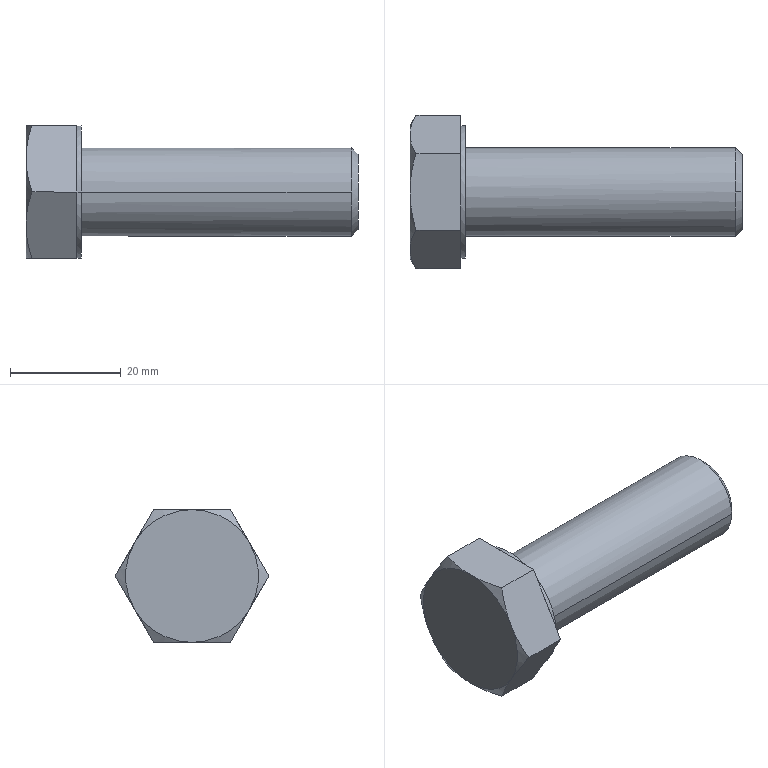Part | SolidWorks | features BaseBody 1 | 1 solid | 27 faces | box 60 x 27.713 x 24 mm | volume 14953 mm3 | plane 15 | cone 8 | cylinder 4 | commonest cylinder face diameters 16 x2 24 x2
STEP:
#1=CARTESIAN_POINT('',(0.,8.,0.));
#2=VERTEX_POINT('',#1);
#3=CARTESIAN_POINT('',(0.,-8.,0.));
#4=VERTEX_POINT('',#3);
#5=CARTESIAN_POINT('',(0.,0.,0.));
#6=DIRECTION('',(1.,0.,0.));
#7=DIRECTION('',(0.,1.,0.));
#8=AXIS2_PLACEMENT_3D('',#5,#6,#7);
#9=CIRCLE('',#8,8.);
#10=EDGE_CURVE('',#2,#4,#9,.T.);
#11=ORIENTED_EDGE('',*,*,#10,.T.);
#12=CARTESIAN_POINT('',(48.773,-8.,0.));
#13=VERTEX_POINT('',#12);
#14=CARTESIAN_POINT('',(28.,-8.,0.));
#15=DIRECTION('',(1.,0.,0.));
#16=VECTOR('',#15,1000.);
#17=LINE('',#14,#16);
#18=EDGE_CURVE('',#4,#13,#17,.T.);
#19=ORIENTED_EDGE('',*,*,#18,.T.);
#20=CARTESIAN_POINT('',(48.773,0.,8.));
#21=VERTEX_POINT('',#20);
#22=CARTESIAN_POINT('',(48.773,0.,0.));
#23=DIRECTION('',(-1.,0.,0.));
#24=DIRECTION('',(0.,1.,0.));
#25=AXIS2_PLACEMENT_3D('',#22,#23,#24);
#26=CIRCLE('',#25,8.);
#27=EDGE_CURVE('',#13,#21,#26,.T.);
#28=ORIENTED_EDGE('',*,*,#27,.T.);
#29=CARTESIAN_POINT('',(48.773,8.,0.));
#30=VERTEX_POINT('',#29);
#31=CARTESIAN_POINT('',(48.773,0.,0.));
#32=DIRECTION('',(-1.,0.,0.));
#33=DIRECTION('',(0.,1.,0.));
#34=AXIS2_PLACEMENT_3D('',#31,#32,#33);
#35=CIRCLE('',#34,8.);
#36=EDGE_CURVE('',#21,#30,#35,.T.);
#37=ORIENTED_EDGE('',*,*,#36,.T.);
#38=CARTESIAN_POINT('',(28.,8.,0.));
#39=DIRECTION('',(1.,0.,0.));
#40=VECTOR('',#39,1000.);
#41=LINE('',#38,#40);
#42=EDGE_CURVE('',#2,#30,#41,.T.);
#43=ORIENTED_EDGE('',*,*,#42,.F.);
#44=EDGE_LOOP('',(#11,#19,#28,#37,#43));
#45=FACE_OUTER_BOUND('',#44,.T.);
#46=CARTESIAN_POINT('',(28.,0.,0.));
#47=DIRECTION('',(1.,0.,0.));
#48=DIRECTION('',(0.,1.,0.));
#49=AXIS2_PLACEMENT_3D('',#46,#47,#48);
#50=CYLINDRICAL_SURFACE('',#49,8.);
#51=ADVANCED_FACE('',(#45),#50,.T.);
#52=CARTESIAN_POINT('',(50.,0.,6.773));
#53=VERTEX_POINT('',#52);
#54=CARTESIAN_POINT('',(50.,0.,-6.773));
#55=VERTEX_POINT('',#54);
#56=CARTESIAN_POINT('',(50.,0.,0.));
#57=DIRECTION('',(-1.,0.,0.));
#58=DIRECTION('',(0.,0.,1.));
#59=AXIS2_PLACEMENT_3D('',#56,#57,#58);
#60=CIRCLE('',#59,6.773);
#61=EDGE_CURVE('',#53,#55,#60,.T.);
#62=ORIENTED_EDGE('',*,*,#61,.T.);
#63=CARTESIAN_POINT('',(48.773,0.,-8.));
#64=VERTEX_POINT('',#63);
#65=CARTESIAN_POINT('',(48.773,0.,-8.));
#66=DIRECTION('',(-0.7071,0.,-0.7071));
#67=VECTOR('',#66,1000.);
#68=LINE('',#65,#67);
#69=EDGE_CURVE('',#55,#64,#68,.T.);
#70=ORIENTED_EDGE('',*,*,#69,.T.);
#71=CARTESIAN_POINT('',(48.773,0.,0.));
#72=DIRECTION('',(-1.,0.,0.));
#73=DIRECTION('',(0.,1.,0.));
#74=AXIS2_PLACEMENT_3D('',#71,#72,#73);
#75=CIRCLE('',#74,8.);
#76=EDGE_CURVE('',#30,#64,#75,.T.);
#77=ORIENTED_EDGE('',*,*,#76,.F.);
#78=ORIENTED_EDGE('',*,*,#36,.F.);
#79=CARTESIAN_POINT('',(48.773,0.,8.));
#80=DIRECTION('',(-0.7071,0.,0.7071));
#81=VECTOR('',#80,1000.);
#82=LINE('',#79,#81);
#83=EDGE_CURVE('',#53,#21,#82,.T.);
#84=ORIENTED_EDGE('',*,*,#83,.F.);
#85=EDGE_LOOP('',(#62,#70,#77,#78,#84));
#86=FACE_OUTER_BOUND('',#85,.T.);
#87=CARTESIAN_POINT('',(48.773,0.,0.));
#88=DIRECTION('',(-1.,0.,0.));
#89=DIRECTION('',(0.,0.,1.));
#90=AXIS2_PLACEMENT_3D('',#87,#88,#89);
#91=CONICAL_SURFACE('',#90,8.,0.7854);
#92=ADVANCED_FACE('',(#86),#91,.T.);
#93=CARTESIAN_POINT('',(-0.8001,-10.392,6.));
#94=VERTEX_POINT('',#93);
#95=CARTESIAN_POINT('',(-0.8001,-12.,0.));
#96=VERTEX_POINT('',#95);
#97=CARTESIAN_POINT('',(-0.8001,0.,0.));
#98=DIRECTION('',(1.,0.,0.));
#99=DIRECTION('',(0.,1.,0.));
#100=AXIS2_PLACEMENT_3D('',#97,#98,#99);
#101=CIRCLE('',#100,12.);
#102=EDGE_CURVE('',#94,#96,#101,.T.);
#103=ORIENTED_EDGE('',*,*,#102,.T.);
#104=CARTESIAN_POINT('',(0.,-12.,0.));
#105=VERTEX_POINT('',#104);
#106=CARTESIAN_POINT('',(-0.4,-12.,0.));
#107=DIRECTION('',(1.,0.,0.));
#108=VECTOR('',#107,1000.);
#109=LINE('',#106,#108);
#110=EDGE_CURVE('',#96,#105,#109,.T.);
#111=ORIENTED_EDGE('',*,*,#110,.T.);
#112=CARTESIAN_POINT('',(0.,12.,0.));
#113=VERTEX_POINT('',#112);
#114=CARTESIAN_POINT('',(0.,0.,0.));
#115=DIRECTION('',(1.,0.,0.));
#116=DIRECTION('',(0.,1.,0.));
#117=AXIS2_PLACEMENT_3D('',#114,#115,#116);
#118=CIRCLE('',#117,12.);
#119=EDGE_CURVE('',#113,#105,#118,.T.);
#120=ORIENTED_EDGE('',*,*,#119,.F.);
#121=CARTESIAN_POINT('',(-0.8001,12.,0.));
#122=VERTEX_POINT('',#121);
#123=CARTESIAN_POINT('',(-0.4,12.,0.));
#124=DIRECTION('',(1.,0.,0.));
#125=VECTOR('',#124,1000.);
#126=LINE('',#123,#125);
#127=EDGE_CURVE('',#122,#113,#126,.T.);
#128=ORIENTED_EDGE('',*,*,#127,.F.);
#129=CARTESIAN_POINT('',(-0.8001,10.392,6.));
#130=VERTEX_POINT('',#129);
#131=CARTESIAN_POINT('',(-0.8001,0.,0.));
#132=DIRECTION('',(1.,0.,0.));
#133=DIRECTION('',(0.,1.,0.));
#134=AXIS2_PLACEMENT_3D('',#131,#132,#133);
#135=CIRCLE('',#134,12.);
#136=EDGE_CURVE('',#122,#130,#135,.T.);
#137=ORIENTED_EDGE('',*,*,#136,.T.);
#138=CARTESIAN_POINT('',(-0.8001,0.,12.));
#139=VERTEX_POINT('',#138);
#140=CARTESIAN_POINT('',(-0.8001,0.,0.));
#141=DIRECTION('',(1.,0.,0.));
#142=DIRECTION('',(0.,1.,0.));
#143=AXIS2_PLACEMENT_3D('',#140,#141,#142);
#144=CIRCLE('',#143,12.);
#145=EDGE_CURVE('',#130,#139,#144,.T.);
#146=ORIENTED_EDGE('',*,*,#145,.T.);
#147=CARTESIAN_POINT('',(-0.8001,0.,0.));
#148=DIRECTION('',(1.,0.,0.));
#149=DIRECTION('',(0.,1.,0.));
#150=AXIS2_PLACEMENT_3D('',#147,#148,#149);
#151=CIRCLE('',#150,12.);
#152=EDGE_CURVE('',#139,#94,#151,.T.);
#153=ORIENTED_EDGE('',*,*,#152,.T.);
#154=EDGE_LOOP('',(#103,#111,#120,#128,#137,#146,#153));
#155=FACE_OUTER_BOUND('',#154,.T.);
#156=CARTESIAN_POINT('',(-0.4,0.,0.));
#157=DIRECTION('',(1.,0.,0.));
#158=DIRECTION('',(0.,1.,0.));
#159=AXIS2_PLACEMENT_3D('',#156,#157,#158);
#160=CYLINDRICAL_SURFACE('',#159,12.);
#161=ADVANCED_FACE('',(#155),#160,.T.);
#162=ORIENTED_EDGE('',*,*,#18,.F.);
#163=CARTESIAN_POINT('',(0.,0.,0.));
#164=DIRECTION('',(1.,0.,0.));
#165=DIRECTION('',(0.,1.,0.));
#166=AXIS2_PLACEMENT_3D('',#163,#164,#165);
#167=CIRCLE('',#166,8.);
#168=EDGE_CURVE('',#4,#2,#167,.T.);
#169=ORIENTED_EDGE('',*,*,#168,.T.);
#170=ORIENTED_EDGE('',*,*,#42,.T.);
#171=ORIENTED_EDGE('',*,*,#76,.T.);
#172=CARTESIAN_POINT('',(48.773,0.,0.));
#173=DIRECTION('',(-1.,0.,0.));
#174=DIRECTION('',(0.,1.,0.));
#175=AXIS2_PLACEMENT_3D('',#172,#173,#174);
#176=CIRCLE('',#175,8.);
#177=EDGE_CURVE('',#64,#13,#176,.T.);
#178=ORIENTED_EDGE('',*,*,#177,.T.);
#179=EDGE_LOOP('',(#162,#169,#170,#171,#178));
#180=FACE_OUTER_BOUND('',#179,.T.);
#181=CARTESIAN_POINT('',(28.,0.,0.));
#182=DIRECTION('',(1.,0.,0.));
#183=DIRECTION('',(0.,1.,0.));
#184=AXIS2_PLACEMENT_3D('',#181,#182,#183);
#185=CYLINDRICAL_SURFACE('',#184,8.);
#186=ADVANCED_FACE('',(#180),#185,.T.);
#187=ORIENTED_EDGE('',*,*,#69,.F.);
#188=CARTESIAN_POINT('',(50.,0.,0.));
#189=DIRECTION('',(-1.,0.,0.));
#190=DIRECTION('',(0.,0.,1.));
#191=AXIS2_PLACEMENT_3D('',#188,#189,#190);
#192=CIRCLE('',#191,6.773);
#193=EDGE_CURVE('',#55,#53,#192,.T.);
#194=ORIENTED_EDGE('',*,*,#193,.T.);
#195=ORIENTED_EDGE('',*,*,#83,.T.);
#196=ORIENTED_EDGE('',*,*,#27,.F.);
#197=ORIENTED_EDGE('',*,*,#177,.F.);
#198=EDGE_LOOP('',(#187,#194,#195,#196,#197));
#199=FACE_OUTER_BOUND('',#198,.T.);
#200=CARTESIAN_POINT('',(48.773,0.,0.));
#201=DIRECTION('',(-1.,0.,0.));
#202=DIRECTION('',(0.,0.,1.));
#203=AXIS2_PLACEMENT_3D('',#200,#201,#202);
#204=CONICAL_SURFACE('',#203,8.,0.7854);
#205=ADVANCED_FACE('',(#199),#204,.T.);
#206=ORIENTED_EDGE('',*,*,#10,.F.);
#207=ORIENTED_EDGE('',*,*,#168,.F.);
#208=EDGE_LOOP('',(#206,#207));
#209=FACE_BOUND('',#208,.T.);
#210=ORIENTED_EDGE('',*,*,#119,.T.);
#211=CARTESIAN_POINT('',(0.,0.,0.));
#212=DIRECTION('',(1.,0.,0.));
#213=DIRECTION('',(0.,1.,0.));
#214=AXIS2_PLACEMENT_3D('',#211,#212,#213);
#215=CIRCLE('',#214,12.);
#216=EDGE_CURVE('',#105,#113,#215,.T.);
#217=ORIENTED_EDGE('',*,*,#216,.T.);
#218=EDGE_LOOP('',(#210,#217));
#219=FACE_OUTER_BOUND('',#218,.T.);
#220=CARTESIAN_POINT('',(0.,10.,0.));
#221=DIRECTION('',(1.,0.,0.));
#222=DIRECTION('',(0.,1.,0.));
#223=AXIS2_PLACEMENT_3D('',#220,#221,#222);
#224=PLANE('',#223);
#225=ADVANCED_FACE('',(#209,#219),#224,.T.);
#226=ORIENTED_EDGE('',*,*,#61,.F.);
#227=ORIENTED_EDGE('',*,*,#193,.F.);
#228=EDGE_LOOP('',(#226,#227));
#229=FACE_OUTER_BOUND('',#228,.T.);
#230=CARTESIAN_POINT('',(50.,4.,0.));
#231=DIRECTION('',(1.,0.,0.));
#232=DIRECTION('',(0.,1.,0.));
#233=AXIS2_PLACEMENT_3D('',#230,#231,#232);
#234=PLANE('',#233);
#235=ADVANCED_FACE('',(#229),#234,.T.);
#236=ORIENTED_EDGE('',*,*,#110,.F.);
#237=CARTESIAN_POINT('',(-0.8001,-10.392,-6.));
#238=VERTEX_POINT('',#237);
#239=CARTESIAN_POINT('',(-0.8001,0.,0.));
#240=DIRECTION('',(1.,0.,0.));
#241=DIRECTION('',(0.,1.,0.));
#242=AXIS2_PLACEMENT_3D('',#239,#240,#241);
#243=CIRCLE('',#242,12.);
#244=EDGE_CURVE('',#96,#238,#243,.T.);
#245=ORIENTED_EDGE('',*,*,#244,.T.);
#246=CARTESIAN_POINT('',(-0.8001,0.,-12.));
#247=VERTEX_POINT('',#246);
#248=CARTESIAN_POINT('',(-0.8001,0.,0.));
#249=DIRECTION('',(1.,0.,0.));
#250=DIRECTION('',(0.,1.,0.));
#251=AXIS2_PLACEMENT_3D('',#248,#249,#250);
#252=CIRCLE('',#251,12.);
#253=EDGE_CURVE('',#238,#247,#252,.T.);
#254=ORIENTED_EDGE('',*,*,#253,.T.);
#255=CARTESIAN_POINT('',(-0.8001,10.392,-6.));
#256=VERTEX_POINT('',#255);
#257=CARTESIAN_POINT('',(-0.8001,0.,0.));
#258=DIRECTION('',(1.,0.,0.));
#259=DIRECTION('',(0.,1.,0.));
#260=AXIS2_PLACEMENT_3D('',#257,#258,#259);
#261=CIRCLE('',#260,12.);
#262=EDGE_CURVE('',#247,#256,#261,.T.);
#263=ORIENTED_EDGE('',*,*,#262,.T.);
#264=CARTESIAN_POINT('',(-0.8001,0.,0.));
#265=DIRECTION('',(1.,0.,0.));
#266=DIRECTION('',(0.,1.,0.));
#267=AXIS2_PLACEMENT_3D('',#264,#265,#266);
#268=CIRCLE('',#267,12.);
#269=EDGE_CURVE('',#256,#122,#268,.T.);
#270=ORIENTED_EDGE('',*,*,#269,.T.);
#271=ORIENTED_EDGE('',*,*,#127,.T.);
#272=ORIENTED_EDGE('',*,*,#216,.F.);
#273=EDGE_LOOP('',(#236,#245,#254,#263,#270,#271,#272));
#274=FACE_OUTER_BOUND('',#273,.T.);
#275=CARTESIAN_POINT('',(-0.4,0.,0.));
#276=DIRECTION('',(1.,0.,0.));
#277=DIRECTION('',(0.,1.,0.));
#278=AXIS2_PLACEMENT_3D('',#275,#276,#277);
#279=CYLINDRICAL_SURFACE('',#278,12.);
#280=ADVANCED_FACE('',(#274),#279,.T.);
#281=CARTESIAN_POINT('',(-0.8001,6.928,-12.));
#282=VERTEX_POINT('',#281);
#283=CARTESIAN_POINT('',(-0.8001,0.,-12.));
#284=DIRECTION('',(0.,1.,0.));
#285=VECTOR('',#284,1000.);
#286=LINE('',#283,#285);
#287=EDGE_CURVE('',#247,#282,#286,.T.);
#288=ORIENTED_EDGE('',*,*,#287,.T.);
#289=CARTESIAN_POINT('',(-0.8001,6.928,-12.));
#290=DIRECTION('',(0.,0.5,0.866));
#291=VECTOR('',#290,1000.);
#292=LINE('',#289,#291);
#293=EDGE_CURVE('',#282,#256,#292,.T.);
#294=ORIENTED_EDGE('',*,*,#293,.T.);
#295=ORIENTED_EDGE('',*,*,#262,.F.);
#296=EDGE_LOOP('',(#288,#294,#295));
#297=FACE_OUTER_BOUND('',#296,.T.);
#298=CARTESIAN_POINT('',(-0.8001,0.,0.));
#299=DIRECTION('',(1.,0.,0.));
#300=DIRECTION('',(0.,1.,0.));
#301=AXIS2_PLACEMENT_3D('',#298,#299,#300);
#302=PLANE('',#301);
#303=ADVANCED_FACE('',(#297),#302,.T.);
#304=CARTESIAN_POINT('',(-0.8001,-6.928,-12.));
#305=VERTEX_POINT('',#304);
#306=CARTESIAN_POINT('',(-0.8001,-10.392,-6.));
#307=DIRECTION('',(0.,0.5,-0.866));
#308=VECTOR('',#307,1000.);
#309=LINE('',#306,#308);
#310=EDGE_CURVE('',#238,#305,#309,.T.);
#311=ORIENTED_EDGE('',*,*,#310,.T.);
#312=CARTESIAN_POINT('',(-0.8001,0.,-12.));
#313=DIRECTION('',(0.,1.,0.));
#314=VECTOR('',#313,1000.);
#315=LINE('',#312,#314);
#316=EDGE_CURVE('',#305,#247,#315,.T.);
#317=ORIENTED_EDGE('',*,*,#316,.T.);
#318=ORIENTED_EDGE('',*,*,#253,.F.);
#319=EDGE_LOOP('',(#311,#317,#318));
#320=FACE_OUTER_BOUND('',#319,.T.);
#321=CARTESIAN_POINT('',(-0.8001,0.,0.));
#322=DIRECTION('',(1.,0.,0.));
#323=DIRECTION('',(0.,1.,0.));
#324=AXIS2_PLACEMENT_3D('',#321,#322,#323);
#325=PLANE('',#324);
#326=ADVANCED_FACE('',(#320),#325,.T.);
#327=CARTESIAN_POINT('',(-0.8001,-13.856,0.));
#328=VERTEX_POINT('',#327);
#329=CARTESIAN_POINT('',(-0.8001,-10.392,6.));
#330=DIRECTION('',(0.,-0.5,-0.866));
#331=VECTOR('',#330,1000.);
#332=LINE('',#329,#331);
#333=EDGE_CURVE('',#94,#328,#332,.T.);
#334=ORIENTED_EDGE('',*,*,#333,.T.);
#335=CARTESIAN_POINT('',(-0.8001,-13.856,0.));
#336=DIRECTION('',(0.,0.5,-0.866));
#337=VECTOR('',#336,1000.);
#338=LINE('',#335,#337);
#339=EDGE_CURVE('',#328,#238,#338,.T.);
#340=ORIENTED_EDGE('',*,*,#339,.T.);
#341=ORIENTED_EDGE('',*,*,#244,.F.);
#342=ORIENTED_EDGE('',*,*,#102,.F.);
#343=EDGE_LOOP('',(#334,#340,#341,#342));
#344=FACE_OUTER_BOUND('',#343,.T.);
#345=CARTESIAN_POINT('',(-0.8001,0.,0.));
#346=DIRECTION('',(1.,0.,0.));
#347=DIRECTION('',(0.,1.,0.));
#348=AXIS2_PLACEMENT_3D('',#345,#346,#347);
#349=PLANE('',#348);
#350=ADVANCED_FACE('',(#344),#349,.T.);
#351=CARTESIAN_POINT('',(-0.8001,-6.928,12.));
#352=VERTEX_POINT('',#351);
#353=CARTESIAN_POINT('',(-0.8001,0.,12.));
#354=DIRECTION('',(0.,-1.,0.));
#355=VECTOR('',#354,1000.);
#356=LINE('',#353,#355);
#357=EDGE_CURVE('',#139,#352,#356,.T.);
#358=ORIENTED_EDGE('',*,*,#357,.T.);
#359=CARTESIAN_POINT('',(-0.8001,-6.928,12.));
#360=DIRECTION('',(0.,-0.5,-0.866));
#361=VECTOR('',#360,1000.);
#362=LINE('',#359,#361);
#363=EDGE_CURVE('',#352,#94,#362,.T.);
#364=ORIENTED_EDGE('',*,*,#363,.T.);
#365=ORIENTED_EDGE('',*,*,#152,.F.);
#366=EDGE_LOOP('',(#358,#364,#365));
#367=FACE_OUTER_BOUND('',#366,.T.);
#368=CARTESIAN_POINT('',(-0.8001,0.,0.));
#369=DIRECTION('',(1.,0.,0.));
#370=DIRECTION('',(0.,1.,0.));
#371=AXIS2_PLACEMENT_3D('',#368,#369,#370);
#372=PLANE('',#371);
#373=ADVANCED_FACE('',(#367),#372,.T.);
#374=CARTESIAN_POINT('',(-0.8001,6.928,12.));
#375=VERTEX_POINT('',#374);
#376=CARTESIAN_POINT('',(-0.8001,10.392,6.));
#377=DIRECTION('',(0.,-0.5,0.866));
#378=VECTOR('',#377,1000.);
#379=LINE('',#376,#378);
#380=EDGE_CURVE('',#130,#375,#379,.T.);
#381=ORIENTED_EDGE('',*,*,#380,.T.);
#382=CARTESIAN_POINT('',(-0.8001,0.,12.));
#383=DIRECTION('',(0.,-1.,0.));
#384=VECTOR('',#383,1000.);
#385=LINE('',#382,#384);
#386=EDGE_CURVE('',#375,#139,#385,.T.);
#387=ORIENTED_EDGE('',*,*,#386,.T.);
#388=ORIENTED_EDGE('',*,*,#145,.F.);
#389=EDGE_LOOP('',(#381,#387,#388));
#390=FACE_OUTER_BOUND('',#389,.T.);
#391=CARTESIAN_POINT('',(-0.8001,0.,0.));
#392=DIRECTION('',(1.,0.,0.));
#393=DIRECTION('',(0.,1.,0.));
#394=AXIS2_PLACEMENT_3D('',#391,#392,#393);
#395=PLANE('',#394);
#396=ADVANCED_FACE('',(#390),#395,.T.);
#397=CARTESIAN_POINT('',(-0.8001,13.856,0.));
#398=VERTEX_POINT('',#397);
#399=CARTESIAN_POINT('',(-0.8001,10.392,-6.));
#400=DIRECTION('',(0.,0.5,0.866));
#401=VECTOR('',#400,1000.);
#402=LINE('',#399,#401);
#403=EDGE_CURVE('',#256,#398,#402,.T.);
#404=ORIENTED_EDGE('',*,*,#403,.T.);
#405=CARTESIAN_POINT('',(-0.8001,13.856,0.));
#406=DIRECTION('',(0.,-0.5,0.866));
#407=VECTOR('',#406,1000.);
#408=LINE('',#405,#407);
#409=EDGE_CURVE('',#398,#130,#408,.T.);
#410=ORIENTED_EDGE('',*,*,#409,.T.);
#411=ORIENTED_EDGE('',*,*,#136,.F.);
#412=ORIENTED_EDGE('',*,*,#269,.F.);
#413=EDGE_LOOP('',(#404,#410,#411,#412));
#414=FACE_OUTER_BOUND('',#413,.T.);
#415=CARTESIAN_POINT('',(-0.8001,0.,0.));
#416=DIRECTION('',(1.,0.,0.));
#417=DIRECTION('',(0.,1.,0.));
#418=AXIS2_PLACEMENT_3D('',#415,#416,#417);
#419=PLANE('',#418);
#420=ADVANCED_FACE('',(#414),#419,.T.);
#421=ORIENTED_EDGE('',*,*,#293,.F.);
#422=CARTESIAN_POINT('',(-8.928,6.928,-12.));
#423=VERTEX_POINT('',#422);
#424=CARTESIAN_POINT('',(-0.8001,6.928,-12.));
#425=DIRECTION('',(-1.,0.,0.));
#426=VECTOR('',#425,1000.);
#427=LINE('',#424,#426);
#428=EDGE_CURVE('',#282,#423,#427,.T.);
#429=ORIENTED_EDGE('',*,*,#428,.T.);
#430=CARTESIAN_POINT('',(-10.,10.392,-6.));
#431=VERTEX_POINT('',#430);
#432=CARTESIAN_POINT('',(-8.928,6.928,-12.));
#433=CARTESIAN_POINT('',(-9.255,7.494,-11.02));
#434=CARTESIAN_POINT('',(-9.524,8.064,-10.032));
#435=CARTESIAN_POINT('',(-9.898,9.218,-8.034));
#436=CARTESIAN_POINT('',(-10.,9.801,-7.024));
#437=CARTESIAN_POINT('',(-10.,10.392,-6.));
#438=B_SPLINE_CURVE_WITH_KNOTS('',3,(#432,#433,#434,#435,#436,#437),.UNSPECIFIED.,.F.,.F.,(4,2,4),(0.,0.003505,0.007011),.UNSPECIFIED.);
#439=EDGE_CURVE('',#423,#431,#438,.T.);
#440=ORIENTED_EDGE('',*,*,#439,.T.);
#441=CARTESIAN_POINT('',(-8.928,13.856,0.));
#442=VERTEX_POINT('',#441);
#443=CARTESIAN_POINT('',(-10.,10.392,-6.));
#444=CARTESIAN_POINT('',(-10.,10.983,-4.976));
#445=CARTESIAN_POINT('',(-9.898,11.567,-3.966));
#446=CARTESIAN_POINT('',(-9.524,12.72,-1.968));
#447=CARTESIAN_POINT('',(-9.255,13.291,-0.9802));
#448=CARTESIAN_POINT('',(-8.928,13.856,0.));
#449=B_SPLINE_CURVE_WITH_KNOTS('',3,(#443,#444,#445,#446,#447,#448),.UNSPECIFIED.,.F.,.F.,(4,2,4),(0.,0.003505,0.007011),.UNSPECIFIED.);
#450=EDGE_CURVE('',#431,#442,#449,.T.);
#451=ORIENTED_EDGE('',*,*,#450,.T.);
#452=CARTESIAN_POINT('',(-0.8001,13.856,0.));
#453=DIRECTION('',(1.,0.,0.));
#454=VECTOR('',#453,1000.);
#455=LINE('',#452,#454);
#456=EDGE_CURVE('',#442,#398,#455,.T.);
#457=ORIENTED_EDGE('',*,*,#456,.T.);
#458=ORIENTED_EDGE('',*,*,#403,.F.);
#459=EDGE_LOOP('',(#421,#429,#440,#451,#457,#458));
#460=FACE_OUTER_BOUND('',#459,.T.);
#461=CARTESIAN_POINT('',(-0.8001,6.928,-12.));
#462=DIRECTION('',(0.,0.866,-0.5));
#463=DIRECTION('',(0.,0.5,0.866));
#464=AXIS2_PLACEMENT_3D('',#461,#462,#463);
#465=PLANE('',#464);
#466=ADVANCED_FACE('',(#460),#465,.T.);
#467=ORIENTED_EDGE('',*,*,#316,.F.);
#468=CARTESIAN_POINT('',(-8.928,-6.928,-12.));
#469=VERTEX_POINT('',#468);
#470=CARTESIAN_POINT('',(-0.8001,-6.928,-12.));
#471=DIRECTION('',(-1.,0.,0.));
#472=VECTOR('',#471,1000.);
#473=LINE('',#470,#472);
#474=EDGE_CURVE('',#305,#469,#473,.T.);
#475=ORIENTED_EDGE('',*,*,#474,.T.);
#476=CARTESIAN_POINT('',(-10.,0.,-12.));
#477=VERTEX_POINT('',#476);
#478=CARTESIAN_POINT('',(-8.928,-6.928,-12.));
#479=CARTESIAN_POINT('',(-9.255,-5.796,-12.));
#480=CARTESIAN_POINT('',(-9.524,-4.656,-12.));
#481=CARTESIAN_POINT('',(-9.898,-2.349,-12.));
#482=CARTESIAN_POINT('',(-10.,-1.182,-12.));
#483=CARTESIAN_POINT('',(-10.,0.,-12.));
#484=B_SPLINE_CURVE_WITH_KNOTS('',3,(#478,#479,#480,#481,#482,#483),.UNSPECIFIED.,.F.,.F.,(4,2,4),(0.,0.003505,0.007011),.UNSPECIFIED.);
#485=EDGE_CURVE('',#469,#477,#484,.T.);
#486=ORIENTED_EDGE('',*,*,#485,.T.);
#487=CARTESIAN_POINT('',(-10.,0.,-12.));
#488=CARTESIAN_POINT('',(-10.,1.182,-12.));
#489=CARTESIAN_POINT('',(-9.898,2.349,-12.));
#490=CARTESIAN_POINT('',(-9.524,4.656,-12.));
#491=CARTESIAN_POINT('',(-9.255,5.796,-12.));
#492=CARTESIAN_POINT('',(-8.928,6.928,-12.));
#493=B_SPLINE_CURVE_WITH_KNOTS('',3,(#487,#488,#489,#490,#491,#492),.UNSPECIFIED.,.F.,.F.,(4,2,4),(0.,0.003505,0.007011),.UNSPECIFIED.);
#494=EDGE_CURVE('',#477,#423,#493,.T.);
#495=ORIENTED_EDGE('',*,*,#494,.T.);
#496=ORIENTED_EDGE('',*,*,#428,.F.);
#497=ORIENTED_EDGE('',*,*,#287,.F.);
#498=EDGE_LOOP('',(#467,#475,#486,#495,#496,#497));
#499=FACE_OUTER_BOUND('',#498,.T.);
#500=CARTESIAN_POINT('',(-0.8001,-6.928,-12.));
#501=DIRECTION('',(0.,0.,-1.));
#502=DIRECTION('',(0.,1.,0.));
#503=AXIS2_PLACEMENT_3D('',#500,#501,#502);
#504=PLANE('',#503);
#505=ADVANCED_FACE('',(#499),#504,.T.);
#506=CARTESIAN_POINT('',(-8.928,-13.856,0.));
#507=VERTEX_POINT('',#506);
#508=CARTESIAN_POINT('',(-0.8001,-13.856,0.));
#509=DIRECTION('',(-1.,0.,0.));
#510=VECTOR('',#509,1000.);
#511=LINE('',#508,#510);
#512=EDGE_CURVE('',#328,#507,#511,.T.);
#513=ORIENTED_EDGE('',*,*,#512,.T.);
#514=CARTESIAN_POINT('',(-10.,-10.392,-6.));
#515=VERTEX_POINT('',#514);
#516=CARTESIAN_POINT('',(-8.928,-13.856,0.));
#517=CARTESIAN_POINT('',(-9.255,-13.291,-0.9802));
#518=CARTESIAN_POINT('',(-9.524,-12.72,-1.968));
#519=CARTESIAN_POINT('',(-9.898,-11.567,-3.966));
#520=CARTESIAN_POINT('',(-10.,-10.983,-4.976));
#521=CARTESIAN_POINT('',(-10.,-10.392,-6.));
#522=B_SPLINE_CURVE_WITH_KNOTS('',3,(#516,#517,#518,#519,#520,#521),.UNSPECIFIED.,.F.,.F.,(4,2,4),(0.,0.003505,0.007011),.UNSPECIFIED.);
#523=EDGE_CURVE('',#507,#515,#522,.T.);
#524=ORIENTED_EDGE('',*,*,#523,.T.);
#525=CARTESIAN_POINT('',(-10.,-10.392,-6.));
#526=CARTESIAN_POINT('',(-10.,-9.801,-7.024));
#527=CARTESIAN_POINT('',(-9.898,-9.218,-8.034));
#528=CARTESIAN_POINT('',(-9.524,-8.064,-10.032));
#529=CARTESIAN_POINT('',(-9.255,-7.494,-11.02));
#530=CARTESIAN_POINT('',(-8.928,-6.928,-12.));
#531=B_SPLINE_CURVE_WITH_KNOTS('',3,(#525,#526,#527,#528,#529,#530),.UNSPECIFIED.,.F.,.F.,(4,2,4),(0.,0.003505,0.007011),.UNSPECIFIED.);
#532=EDGE_CURVE('',#515,#469,#531,.T.);
#533=ORIENTED_EDGE('',*,*,#532,.T.);
#534=ORIENTED_EDGE('',*,*,#474,.F.);
#535=ORIENTED_EDGE('',*,*,#310,.F.);
#536=ORIENTED_EDGE('',*,*,#339,.F.);
#537=EDGE_LOOP('',(#513,#524,#533,#534,#535,#536));
#538=FACE_OUTER_BOUND('',#537,.T.);
#539=CARTESIAN_POINT('',(-0.8001,-13.856,0.));
#540=DIRECTION('',(0.,-0.866,-0.5));
#541=DIRECTION('',(0.,0.5,-0.866));
#542=AXIS2_PLACEMENT_3D('',#539,#540,#541);
#543=PLANE('',#542);
#544=ADVANCED_FACE('',(#538),#543,.T.);
#545=CARTESIAN_POINT('',(-8.928,-6.928,12.));
#546=VERTEX_POINT('',#545);
#547=CARTESIAN_POINT('',(-0.8001,-6.928,12.));
#548=DIRECTION('',(-1.,0.,0.));
#549=VECTOR('',#548,1000.);
#550=LINE('',#547,#549);
#551=EDGE_CURVE('',#352,#546,#550,.T.);
#552=ORIENTED_EDGE('',*,*,#551,.T.);
#553=CARTESIAN_POINT('',(-10.,-10.392,6.));
#554=VERTEX_POINT('',#553);
#555=CARTESIAN_POINT('',(-8.928,-6.928,12.));
#556=CARTESIAN_POINT('',(-9.255,-7.494,11.02));
#557=CARTESIAN_POINT('',(-9.524,-8.064,10.032));
#558=CARTESIAN_POINT('',(-9.898,-9.218,8.034));
#559=CARTESIAN_POINT('',(-10.,-9.801,7.024));
#560=CARTESIAN_POINT('',(-10.,-10.392,6.));
#561=B_SPLINE_CURVE_WITH_KNOTS('',3,(#555,#556,#557,#558,#559,#560),.UNSPECIFIED.,.F.,.F.,(4,2,4),(0.,0.003505,0.007011),.UNSPECIFIED.);
#562=EDGE_CURVE('',#546,#554,#561,.T.);
#563=ORIENTED_EDGE('',*,*,#562,.T.);
#564=CARTESIAN_POINT('',(-10.,-10.392,6.));
#565=CARTESIAN_POINT('',(-10.,-10.983,4.976));
#566=CARTESIAN_POINT('',(-9.898,-11.567,3.966));
#567=CARTESIAN_POINT('',(-9.524,-12.72,1.968));
#568=CARTESIAN_POINT('',(-9.255,-13.291,0.9802));
#569=CARTESIAN_POINT('',(-8.928,-13.856,0.));
#570=B_SPLINE_CURVE_WITH_KNOTS('',3,(#564,#565,#566,#567,#568,#569),.UNSPECIFIED.,.F.,.F.,(4,2,4),(0.,0.003505,0.007011),.UNSPECIFIED.);
#571=EDGE_CURVE('',#554,#507,#570,.T.);
#572=ORIENTED_EDGE('',*,*,#571,.T.);
#573=ORIENTED_EDGE('',*,*,#512,.F.);
#574=ORIENTED_EDGE('',*,*,#333,.F.);
#575=ORIENTED_EDGE('',*,*,#363,.F.);
#576=EDGE_LOOP('',(#552,#563,#572,#573,#574,#575));
#577=FACE_OUTER_BOUND('',#576,.T.);
#578=CARTESIAN_POINT('',(-0.8001,-6.928,12.));
#579=DIRECTION('',(0.,-0.866,0.5));
#580=DIRECTION('',(0.,-0.5,-0.866));
#581=AXIS2_PLACEMENT_3D('',#578,#579,#580);
#582=PLANE('',#581);
#583=ADVANCED_FACE('',(#577),#582,.T.);
#584=CARTESIAN_POINT('',(-8.928,6.928,12.));
#585=VERTEX_POINT('',#584);
#586=CARTESIAN_POINT('',(-0.8001,6.928,12.));
#587=DIRECTION('',(-1.,0.,0.));
#588=VECTOR('',#587,1000.);
#589=LINE('',#586,#588);
#590=EDGE_CURVE('',#375,#585,#589,.T.);
#591=ORIENTED_EDGE('',*,*,#590,.T.);
#592=CARTESIAN_POINT('',(-10.,0.,12.));
#593=VERTEX_POINT('',#592);
#594=CARTESIAN_POINT('',(-8.928,6.928,12.));
#595=CARTESIAN_POINT('',(-9.255,5.796,12.));
#596=CARTESIAN_POINT('',(-9.524,4.656,12.));
#597=CARTESIAN_POINT('',(-9.898,2.349,12.));
#598=CARTESIAN_POINT('',(-10.,1.182,12.));
#599=CARTESIAN_POINT('',(-10.,0.,12.));
#600=B_SPLINE_CURVE_WITH_KNOTS('',3,(#594,#595,#596,#597,#598,#599),.UNSPECIFIED.,.F.,.F.,(4,2,4),(0.,0.003505,0.007011),.UNSPECIFIED.);
#601=EDGE_CURVE('',#585,#593,#600,.T.);
#602=ORIENTED_EDGE('',*,*,#601,.T.);
#603=CARTESIAN_POINT('',(-10.,0.,12.));
#604=CARTESIAN_POINT('',(-10.,-1.182,12.));
#605=CARTESIAN_POINT('',(-9.898,-2.349,12.));
#606=CARTESIAN_POINT('',(-9.524,-4.656,12.));
#607=CARTESIAN_POINT('',(-9.255,-5.796,12.));
#608=CARTESIAN_POINT('',(-8.928,-6.928,12.));
#609=B_SPLINE_CURVE_WITH_KNOTS('',3,(#603,#604,#605,#606,#607,#608),.UNSPECIFIED.,.F.,.F.,(4,2,4),(0.,0.003505,0.007011),.UNSPECIFIED.);
#610=EDGE_CURVE('',#593,#546,#609,.T.);
#611=ORIENTED_EDGE('',*,*,#610,.T.);
#612=ORIENTED_EDGE('',*,*,#551,.F.);
#613=ORIENTED_EDGE('',*,*,#357,.F.);
#614=ORIENTED_EDGE('',*,*,#386,.F.);
#615=EDGE_LOOP('',(#591,#602,#611,#612,#613,#614));
#616=FACE_OUTER_BOUND('',#615,.T.);
#617=CARTESIAN_POINT('',(-0.8001,6.928,12.));
#618=DIRECTION('',(0.,0.,1.));
#619=DIRECTION('',(0.,-1.,0.));
#620=AXIS2_PLACEMENT_3D('',#617,#618,#619);
#621=PLANE('',#620);
#622=ADVANCED_FACE('',(#616),#621,.T.);
#623=ORIENTED_EDGE('',*,*,#409,.F.);
#624=ORIENTED_EDGE('',*,*,#456,.F.);
#625=CARTESIAN_POINT('',(-10.,10.392,6.));
#626=VERTEX_POINT('',#625);
#627=CARTESIAN_POINT('',(-8.928,13.856,0.));
#628=CARTESIAN_POINT('',(-9.255,13.291,0.9802));
#629=CARTESIAN_POINT('',(-9.524,12.72,1.968));
#630=CARTESIAN_POINT('',(-9.898,11.567,3.966));
#631=CARTESIAN_POINT('',(-10.,10.983,4.976));
#632=CARTESIAN_POINT('',(-10.,10.392,6.));
#633=B_SPLINE_CURVE_WITH_KNOTS('',3,(#627,#628,#629,#630,#631,#632),.UNSPECIFIED.,.F.,.F.,(4,2,4),(0.,0.003505,0.007011),.UNSPECIFIED.);
#634=EDGE_CURVE('',#442,#626,#633,.T.);
#635=ORIENTED_EDGE('',*,*,#634,.T.);
#636=CARTESIAN_POINT('',(-10.,10.392,6.));
#637=CARTESIAN_POINT('',(-10.,9.801,7.024));
#638=CARTESIAN_POINT('',(-9.898,9.218,8.034));
#639=CARTESIAN_POINT('',(-9.524,8.064,10.032));
#640=CARTESIAN_POINT('',(-9.255,7.494,11.02));
#641=CARTESIAN_POINT('',(-8.928,6.928,12.));
#642=B_SPLINE_CURVE_WITH_KNOTS('',3,(#636,#637,#638,#639,#640,#641),.UNSPECIFIED.,.F.,.F.,(4,2,4),(0.,0.003505,0.007011),.UNSPECIFIED.);
#643=EDGE_CURVE('',#626,#585,#642,.T.);
#644=ORIENTED_EDGE('',*,*,#643,.T.);
#645=ORIENTED_EDGE('',*,*,#590,.F.);
#646=ORIENTED_EDGE('',*,*,#380,.F.);
#647=EDGE_LOOP('',(#623,#624,#635,#644,#645,#646));
#648=FACE_OUTER_BOUND('',#647,.T.);
#649=CARTESIAN_POINT('',(-0.8001,13.856,0.));
#650=DIRECTION('',(0.,0.866,0.5));
#651=DIRECTION('',(0.,-0.5,0.866));
#652=AXIS2_PLACEMENT_3D('',#649,#650,#651);
#653=PLANE('',#652);
#654=ADVANCED_FACE('',(#648),#653,.T.);
#655=CARTESIAN_POINT('',(-10.,0.,0.));
#656=DIRECTION('',(1.,0.,0.));
#657=DIRECTION('',(0.,0.,-1.));
#658=AXIS2_PLACEMENT_3D('',#655,#656,#657);
#659=CIRCLE('',#658,12.);
#660=EDGE_CURVE('',#431,#626,#659,.T.);
#661=ORIENTED_EDGE('',*,*,#660,.T.);
#662=ORIENTED_EDGE('',*,*,#634,.F.);
#663=ORIENTED_EDGE('',*,*,#450,.F.);
#664=EDGE_LOOP('',(#661,#662,#663));
#665=FACE_OUTER_BOUND('',#664,.T.);
#666=CARTESIAN_POINT('',(-8.922,0.,0.));
#667=DIRECTION('',(1.,0.,0.));
#668=DIRECTION('',(0.,0.,-1.));
#669=AXIS2_PLACEMENT_3D('',#666,#667,#668);
#670=CONICAL_SURFACE('',#669,13.868,1.047);
#671=ADVANCED_FACE('',(#665),#670,.T.);
#672=CARTESIAN_POINT('',(-10.,0.,0.));
#673=DIRECTION('',(1.,0.,0.));
#674=DIRECTION('',(0.,0.,-1.));
#675=AXIS2_PLACEMENT_3D('',#672,#673,#674);
#676=CIRCLE('',#675,12.);
#677=EDGE_CURVE('',#477,#431,#676,.T.);
#678=ORIENTED_EDGE('',*,*,#677,.T.);
#679=ORIENTED_EDGE('',*,*,#439,.F.);
#680=ORIENTED_EDGE('',*,*,#494,.F.);
#681=EDGE_LOOP('',(#678,#679,#680));
#682=FACE_OUTER_BOUND('',#681,.T.);
#683=CARTESIAN_POINT('',(-8.922,0.,0.));
#684=DIRECTION('',(1.,0.,0.));
#685=DIRECTION('',(0.,0.,-1.));
#686=AXIS2_PLACEMENT_3D('',#683,#684,#685);
#687=CONICAL_SURFACE('',#686,13.868,1.047);
#688=ADVANCED_FACE('',(#682),#687,.T.);
#689=ORIENTED_EDGE('',*,*,#532,.F.);
#690=CARTESIAN_POINT('',(-10.,0.,0.));
#691=DIRECTION('',(1.,0.,0.));
#692=DIRECTION('',(0.,0.,-1.));
#693=AXIS2_PLACEMENT_3D('',#690,#691,#692);
#694=CIRCLE('',#693,12.);
#695=EDGE_CURVE('',#515,#477,#694,.T.);
#696=ORIENTED_EDGE('',*,*,#695,.T.);
#697=ORIENTED_EDGE('',*,*,#485,.F.);
#698=EDGE_LOOP('',(#689,#696,#697));
#699=FACE_OUTER_BOUND('',#698,.T.);
#700=CARTESIAN_POINT('',(-8.922,0.,0.));
#701=DIRECTION('',(1.,0.,0.));
#702=DIRECTION('',(0.,0.,-1.));
#703=AXIS2_PLACEMENT_3D('',#700,#701,#702);
#704=CONICAL_SURFACE('',#703,13.868,1.047);
#705=ADVANCED_FACE('',(#699),#704,.T.);
#706=ORIENTED_EDGE('',*,*,#571,.F.);
#707=CARTESIAN_POINT('',(-10.,0.,0.));
#708=DIRECTION('',(1.,0.,0.));
#709=DIRECTION('',(0.,0.,-1.));
#710=AXIS2_PLACEMENT_3D('',#707,#708,#709);
#711=CIRCLE('',#710,12.);
#712=EDGE_CURVE('',#554,#515,#711,.T.);
#713=ORIENTED_EDGE('',*,*,#712,.T.);
#714=ORIENTED_EDGE('',*,*,#523,.F.);
#715=EDGE_LOOP('',(#706,#713,#714));
#716=FACE_OUTER_BOUND('',#715,.T.);
#717=CARTESIAN_POINT('',(-8.922,0.,0.));
#718=DIRECTION('',(1.,0.,0.));
#719=DIRECTION('',(0.,0.,-1.));
#720=AXIS2_PLACEMENT_3D('',#717,#718,#719);
#721=CONICAL_SURFACE('',#720,13.868,1.047);
#722=ADVANCED_FACE('',(#716),#721,.T.);
#723=ORIENTED_EDGE('',*,*,#610,.F.);
#724=CARTESIAN_POINT('',(-10.,0.,0.));
#725=DIRECTION('',(1.,0.,0.));
#726=DIRECTION('',(0.,0.,-1.));
#727=AXIS2_PLACEMENT_3D('',#724,#725,#726);
#728=CIRCLE('',#727,12.);
#729=EDGE_CURVE('',#593,#554,#728,.T.);
#730=ORIENTED_EDGE('',*,*,#729,.T.);
#731=ORIENTED_EDGE('',*,*,#562,.F.);
#732=EDGE_LOOP('',(#723,#730,#731));
#733=FACE_OUTER_BOUND('',#732,.T.);
#734=CARTESIAN_POINT('',(-8.922,0.,0.));
#735=DIRECTION('',(1.,0.,0.));
#736=DIRECTION('',(0.,0.,-1.));
#737=AXIS2_PLACEMENT_3D('',#734,#735,#736);
#738=CONICAL_SURFACE('',#737,13.868,1.047);
#739=ADVANCED_FACE('',(#733),#738,.T.);
#740=CARTESIAN_POINT('',(-10.,0.,0.));
#741=DIRECTION('',(1.,0.,0.));
#742=DIRECTION('',(0.,0.,-1.));
#743=AXIS2_PLACEMENT_3D('',#740,#741,#742);
#744=CIRCLE('',#743,12.);
#745=EDGE_CURVE('',#626,#593,#744,.T.);
#746=ORIENTED_EDGE('',*,*,#745,.T.);
#747=ORIENTED_EDGE('',*,*,#601,.F.);
#748=ORIENTED_EDGE('',*,*,#643,.F.);
#749=EDGE_LOOP('',(#746,#747,#748));
#750=FACE_OUTER_BOUND('',#749,.T.);
#751=CARTESIAN_POINT('',(-8.922,0.,0.));
#752=DIRECTION('',(1.,0.,0.));
#753=DIRECTION('',(0.,0.,-1.));
#754=AXIS2_PLACEMENT_3D('',#751,#752,#753);
#755=CONICAL_SURFACE('',#754,13.868,1.047);
#756=ADVANCED_FACE('',(#750),#755,.T.);
#757=ORIENTED_EDGE('',*,*,#660,.F.);
#758=ORIENTED_EDGE('',*,*,#677,.F.);
#759=ORIENTED_EDGE('',*,*,#695,.F.);
#760=ORIENTED_EDGE('',*,*,#712,.F.);
#761=ORIENTED_EDGE('',*,*,#729,.F.);
#762=ORIENTED_EDGE('',*,*,#745,.F.);
#763=EDGE_LOOP('',(#757,#758,#759,#760,#761,#762));
#764=FACE_OUTER_BOUND('',#763,.T.);
#765=CARTESIAN_POINT('',(-10.,0.,0.));
#766=DIRECTION('',(1.,0.,0.));
#767=DIRECTION('',(0.,1.,0.));
#768=AXIS2_PLACEMENT_3D('',#765,#766,#767);
#769=PLANE('',#768);
#770=ADVANCED_FACE('',(#764),#769,.F.);
#771=CLOSED_SHELL('',(#51,#92,#161,#186,#205,#225,#235,#280,#303,#326,#350,#373,#396,#420,#466,#505,#544,#583,#622,#654,#671,#688,#705,#722,#739,#756,#770));
#772=MANIFOLD_SOLID_BREP('',#771);
#773=CARTESIAN_POINT('',(0.,0.,0.));
#774=DIRECTION('',(0.,0.,1.));
#775=DIRECTION('',(1.,0.,0.));
#776=AXIS2_PLACEMENT_3D('',#773,#774,#775);
#777=(LENGTH_UNIT()NAMED_UNIT(*)SI_UNIT(.MILLI.,.METRE.));
#778=UNCERTAINTY_MEASURE_WITH_UNIT(LENGTH_MEASURE(0.00001),#777,'','');
#779=(NAMED_UNIT(*)PLANE_ANGLE_UNIT()SI_UNIT($,.RADIAN.));
#780=(NAMED_UNIT(*)SI_UNIT($,.STERADIAN.)SOLID_ANGLE_UNIT());
#781=(GEOMETRIC_REPRESENTATION_CONTEXT(3)GLOBAL_UNCERTAINTY_ASSIGNED_CONTEXT((#778))GLOBAL_UNIT_ASSIGNED_CONTEXT((#777,#779,#780))REPRESENTATION_CONTEXT('',''));
#782=ADVANCED_BREP_SHAPE_REPRESENTATION('',(#772,#776),#781);